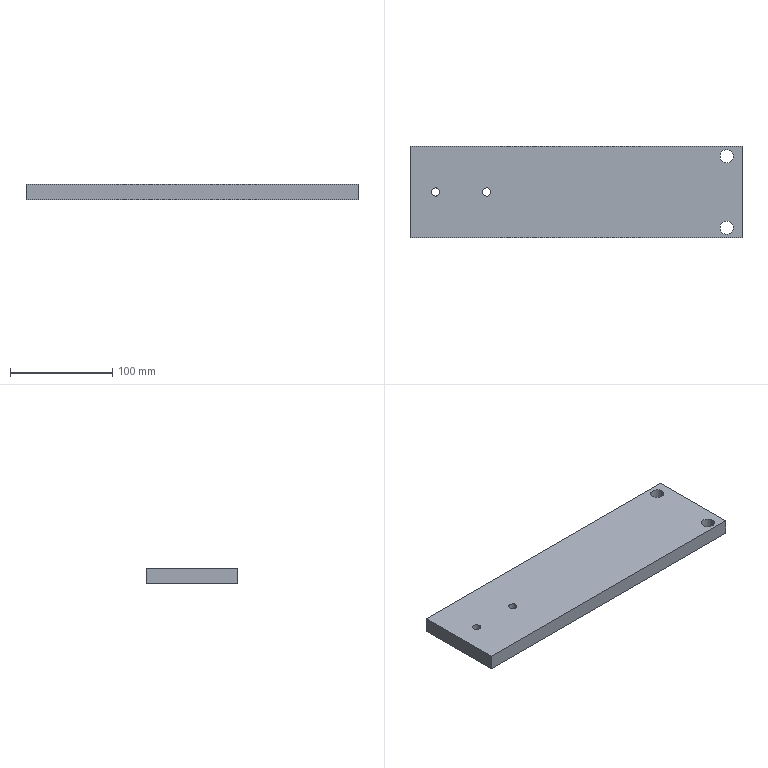Part | NX | features solid 2 | 1 solid | 10 faces | box 325 x 90 x 15 mm | volume 433260 mm3 | plane 6 | cylinder 4 | commonest cylinder face diameters 8 x2 13 x2
STEP:
#1=CARTESIAN_POINT('',(-351.,-440.,-110.));
#2=VERTEX_POINT('',#1);
#3=CARTESIAN_POINT('',(-355.,-440.,-110.));
#4=DIRECTION('',(0.,0.,1.));
#5=DIRECTION('',(1.,0.,0.));
#6=AXIS2_PLACEMENT_3D('',#3,#4,#5);
#7=CIRCLE('',#6,4.);
#8=EDGE_CURVE('',#2,#2,#7,.T.);
#9=ORIENTED_EDGE('',*,*,#8,.F.);
#10=EDGE_LOOP('',(#9));
#11=FACE_BOUND('',#10,.T.);
#12=CARTESIAN_POINT('',(-401.,-440.,-110.));
#13=VERTEX_POINT('',#12);
#14=CARTESIAN_POINT('',(-405.,-440.,-110.));
#15=DIRECTION('',(0.,0.,1.));
#16=DIRECTION('',(1.,0.,0.));
#17=AXIS2_PLACEMENT_3D('',#14,#15,#16);
#18=CIRCLE('',#17,4.);
#19=EDGE_CURVE('',#13,#13,#18,.T.);
#20=ORIENTED_EDGE('',*,*,#19,.F.);
#21=EDGE_LOOP('',(#20));
#22=FACE_BOUND('',#21,.T.);
#23=CARTESIAN_POINT('',(-113.5,-405.,-110.));
#24=VERTEX_POINT('',#23);
#25=CARTESIAN_POINT('',(-120.,-405.,-110.));
#26=DIRECTION('',(0.,0.,1.));
#27=DIRECTION('',(1.,0.,0.));
#28=AXIS2_PLACEMENT_3D('',#25,#26,#27);
#29=CIRCLE('',#28,6.5);
#30=EDGE_CURVE('',#24,#24,#29,.T.);
#31=ORIENTED_EDGE('',*,*,#30,.F.);
#32=EDGE_LOOP('',(#31));
#33=FACE_BOUND('',#32,.T.);
#34=CARTESIAN_POINT('',(-430.,-395.,-110.));
#35=VERTEX_POINT('',#34);
#36=CARTESIAN_POINT('',(-105.,-395.,-110.));
#37=VERTEX_POINT('',#36);
#38=CARTESIAN_POINT('',(-485.,-395.,-110.));
#39=DIRECTION('',(-1.,0.,0.));
#40=VECTOR('',#39,1000.);
#41=LINE('',#38,#40);
#42=EDGE_CURVE('',#35,#37,#41,.F.);
#43=ORIENTED_EDGE('',*,*,#42,.F.);
#44=CARTESIAN_POINT('',(-430.,-485.,-110.));
#45=VERTEX_POINT('',#44);
#46=CARTESIAN_POINT('',(-430.,-395.,-110.));
#47=DIRECTION('',(0.,1.,0.));
#48=VECTOR('',#47,1000.);
#49=LINE('',#46,#48);
#50=EDGE_CURVE('',#45,#35,#49,.T.);
#51=ORIENTED_EDGE('',*,*,#50,.F.);
#52=CARTESIAN_POINT('',(-105.,-485.,-110.));
#53=VERTEX_POINT('',#52);
#54=CARTESIAN_POINT('',(-485.,-485.,-110.));
#55=DIRECTION('',(1.,0.,0.));
#56=VECTOR('',#55,1000.);
#57=LINE('',#54,#56);
#58=EDGE_CURVE('',#45,#53,#57,.T.);
#59=ORIENTED_EDGE('',*,*,#58,.T.);
#60=CARTESIAN_POINT('',(-105.,-775.,-110.));
#61=DIRECTION('',(0.,-1.,0.));
#62=VECTOR('',#61,1000.);
#63=LINE('',#60,#62);
#64=EDGE_CURVE('',#37,#53,#63,.T.);
#65=ORIENTED_EDGE('',*,*,#64,.F.);
#66=EDGE_LOOP('',(#43,#51,#59,#65));
#67=FACE_BOUND('',#66,.T.);
#68=CARTESIAN_POINT('',(-113.5,-475.,-110.));
#69=VERTEX_POINT('',#68);
#70=CARTESIAN_POINT('',(-120.,-475.,-110.));
#71=DIRECTION('',(0.,0.,1.));
#72=DIRECTION('',(1.,0.,0.));
#73=AXIS2_PLACEMENT_3D('',#70,#71,#72);
#74=CIRCLE('',#73,6.5);
#75=EDGE_CURVE('',#69,#69,#74,.F.);
#76=ORIENTED_EDGE('',*,*,#75,.T.);
#77=EDGE_LOOP('',(#76));
#78=FACE_BOUND('',#77,.T.);
#79=CARTESIAN_POINT('',(-485.,-775.,-110.));
#80=DIRECTION('',(0.,0.,1.));
#81=DIRECTION('',(-1.,0.,0.));
#82=AXIS2_PLACEMENT_3D('',#79,#80,#81);
#83=PLANE('',#82);
#84=ADVANCED_FACE('',(#11,#22,#33,#67,#78),#83,.T.);
#85=CARTESIAN_POINT('',(-351.,-440.,-125.));
#86=VERTEX_POINT('',#85);
#87=CARTESIAN_POINT('',(-355.,-440.,-125.));
#88=DIRECTION('',(0.,0.,1.));
#89=DIRECTION('',(1.,0.,0.));
#90=AXIS2_PLACEMENT_3D('',#87,#88,#89);
#91=CIRCLE('',#90,4.);
#92=EDGE_CURVE('',#86,#86,#91,.T.);
#93=ORIENTED_EDGE('',*,*,#92,.T.);
#94=EDGE_LOOP('',(#93));
#95=FACE_BOUND('',#94,.T.);
#96=CARTESIAN_POINT('',(-401.,-440.,-125.));
#97=VERTEX_POINT('',#96);
#98=CARTESIAN_POINT('',(-405.,-440.,-125.));
#99=DIRECTION('',(0.,0.,1.));
#100=DIRECTION('',(1.,0.,0.));
#101=AXIS2_PLACEMENT_3D('',#98,#99,#100);
#102=CIRCLE('',#101,4.);
#103=EDGE_CURVE('',#97,#97,#102,.T.);
#104=ORIENTED_EDGE('',*,*,#103,.T.);
#105=EDGE_LOOP('',(#104));
#106=FACE_BOUND('',#105,.T.);
#107=CARTESIAN_POINT('',(-126.5,-405.,-125.));
#108=VERTEX_POINT('',#107);
#109=CARTESIAN_POINT('',(-120.,-405.,-125.));
#110=DIRECTION('',(0.,0.,-1.));
#111=DIRECTION('',(-1.,0.,0.));
#112=AXIS2_PLACEMENT_3D('',#109,#110,#111);
#113=CIRCLE('',#112,6.5);
#114=EDGE_CURVE('',#108,#108,#113,.F.);
#115=ORIENTED_EDGE('',*,*,#114,.T.);
#116=EDGE_LOOP('',(#115));
#117=FACE_BOUND('',#116,.T.);
#118=CARTESIAN_POINT('',(-105.,-395.,-125.));
#119=VERTEX_POINT('',#118);
#120=CARTESIAN_POINT('',(-105.,-485.,-125.));
#121=VERTEX_POINT('',#120);
#122=CARTESIAN_POINT('',(-105.,-435.,-125.));
#123=DIRECTION('',(0.,1.,0.));
#124=VECTOR('',#123,1000.);
#125=LINE('',#122,#124);
#126=EDGE_CURVE('',#119,#121,#125,.F.);
#127=ORIENTED_EDGE('',*,*,#126,.T.);
#128=CARTESIAN_POINT('',(-430.,-485.,-125.));
#129=VERTEX_POINT('',#128);
#130=CARTESIAN_POINT('',(-135.,-485.,-125.));
#131=DIRECTION('',(-1.,0.,0.));
#132=VECTOR('',#131,1000.);
#133=LINE('',#130,#132);
#134=EDGE_CURVE('',#129,#121,#133,.F.);
#135=ORIENTED_EDGE('',*,*,#134,.F.);
#136=CARTESIAN_POINT('',(-430.,-395.,-125.));
#137=VERTEX_POINT('',#136);
#138=CARTESIAN_POINT('',(-430.,-395.,-125.));
#139=DIRECTION('',(0.,-1.,0.));
#140=VECTOR('',#139,1000.);
#141=LINE('',#138,#140);
#142=EDGE_CURVE('',#129,#137,#141,.F.);
#143=ORIENTED_EDGE('',*,*,#142,.T.);
#144=CARTESIAN_POINT('',(-135.,-395.,-125.));
#145=DIRECTION('',(1.,0.,0.));
#146=VECTOR('',#145,1000.);
#147=LINE('',#144,#146);
#148=EDGE_CURVE('',#137,#119,#147,.T.);
#149=ORIENTED_EDGE('',*,*,#148,.T.);
#150=EDGE_LOOP('',(#127,#135,#143,#149));
#151=FACE_BOUND('',#150,.T.);
#152=CARTESIAN_POINT('',(-126.5,-475.,-125.));
#153=VERTEX_POINT('',#152);
#154=CARTESIAN_POINT('',(-120.,-475.,-125.));
#155=DIRECTION('',(0.,0.,-1.));
#156=DIRECTION('',(-1.,0.,0.));
#157=AXIS2_PLACEMENT_3D('',#154,#155,#156);
#158=CIRCLE('',#157,6.5);
#159=EDGE_CURVE('',#153,#153,#158,.T.);
#160=ORIENTED_EDGE('',*,*,#159,.F.);
#161=EDGE_LOOP('',(#160));
#162=FACE_BOUND('',#161,.T.);
#163=CARTESIAN_POINT('',(-135.,-435.,-125.));
#164=DIRECTION('',(0.,0.,-1.));
#165=DIRECTION('',(0.,-1.,0.));
#166=AXIS2_PLACEMENT_3D('',#163,#164,#165);
#167=PLANE('',#166);
#168=ADVANCED_FACE('',(#95,#106,#117,#151,#162),#167,.T.);
#169=ORIENTED_EDGE('',*,*,#64,.T.);
#170=CARTESIAN_POINT('',(-105.,-485.,-125.));
#171=DIRECTION('',(0.,0.,-1.));
#172=VECTOR('',#171,1000.);
#173=LINE('',#170,#172);
#174=EDGE_CURVE('',#53,#121,#173,.T.);
#175=ORIENTED_EDGE('',*,*,#174,.T.);
#176=ORIENTED_EDGE('',*,*,#126,.F.);
#177=CARTESIAN_POINT('',(-105.,-395.,-125.));
#178=DIRECTION('',(0.,0.,1.));
#179=VECTOR('',#178,1000.);
#180=LINE('',#177,#179);
#181=EDGE_CURVE('',#37,#119,#180,.F.);
#182=ORIENTED_EDGE('',*,*,#181,.F.);
#183=EDGE_LOOP('',(#169,#175,#176,#182));
#184=FACE_BOUND('',#183,.T.);
#185=CARTESIAN_POINT('',(-105.,-395.,-125.));
#186=DIRECTION('',(1.,0.,0.));
#187=DIRECTION('',(0.,0.,1.));
#188=AXIS2_PLACEMENT_3D('',#185,#186,#187);
#189=PLANE('',#188);
#190=ADVANCED_FACE('',(#184),#189,.T.);
#191=ORIENTED_EDGE('',*,*,#181,.T.);
#192=ORIENTED_EDGE('',*,*,#148,.F.);
#193=CARTESIAN_POINT('',(-430.,-395.,-204.));
#194=DIRECTION('',(0.,0.,-1.));
#195=VECTOR('',#194,1000.);
#196=LINE('',#193,#195);
#197=EDGE_CURVE('',#137,#35,#196,.F.);
#198=ORIENTED_EDGE('',*,*,#197,.T.);
#199=ORIENTED_EDGE('',*,*,#42,.T.);
#200=EDGE_LOOP('',(#191,#192,#198,#199));
#201=FACE_BOUND('',#200,.T.);
#202=CARTESIAN_POINT('',(-135.,-395.,-144.));
#203=DIRECTION('',(0.,1.,0.));
#204=DIRECTION('',(0.,0.,-1.));
#205=AXIS2_PLACEMENT_3D('',#202,#203,#204);
#206=PLANE('',#205);
#207=ADVANCED_FACE('',(#201),#206,.T.);
#208=ORIENTED_EDGE('',*,*,#58,.F.);
#209=CARTESIAN_POINT('',(-430.,-485.,-204.));
#210=DIRECTION('',(0.,0.,1.));
#211=VECTOR('',#210,1000.);
#212=LINE('',#209,#211);
#213=EDGE_CURVE('',#129,#45,#212,.T.);
#214=ORIENTED_EDGE('',*,*,#213,.F.);
#215=ORIENTED_EDGE('',*,*,#134,.T.);
#216=ORIENTED_EDGE('',*,*,#174,.F.);
#217=EDGE_LOOP('',(#208,#214,#215,#216));
#218=FACE_BOUND('',#217,.T.);
#219=CARTESIAN_POINT('',(135.,-485.,-144.));
#220=DIRECTION('',(0.,-1.,0.));
#221=DIRECTION('',(0.,0.,1.));
#222=AXIS2_PLACEMENT_3D('',#219,#220,#221);
#223=PLANE('',#222);
#224=ADVANCED_FACE('',(#218),#223,.T.);
#225=ORIENTED_EDGE('',*,*,#213,.T.);
#226=ORIENTED_EDGE('',*,*,#50,.T.);
#227=ORIENTED_EDGE('',*,*,#197,.F.);
#228=ORIENTED_EDGE('',*,*,#142,.F.);
#229=EDGE_LOOP('',(#225,#226,#227,#228));
#230=FACE_BOUND('',#229,.T.);
#231=CARTESIAN_POINT('',(-430.,-395.,-204.));
#232=DIRECTION('',(-1.,0.,0.));
#233=DIRECTION('',(0.,0.,1.));
#234=AXIS2_PLACEMENT_3D('',#231,#232,#233);
#235=PLANE('',#234);
#236=ADVANCED_FACE('',(#230),#235,.T.);
#237=ORIENTED_EDGE('',*,*,#75,.F.);
#238=EDGE_LOOP('',(#237));
#239=FACE_BOUND('',#238,.T.);
#240=ORIENTED_EDGE('',*,*,#159,.T.);
#241=EDGE_LOOP('',(#240));
#242=FACE_BOUND('',#241,.T.);
#243=CARTESIAN_POINT('',(-120.,-475.,-94.));
#244=DIRECTION('',(0.,0.,-1.));
#245=DIRECTION('',(-1.,0.,0.));
#246=AXIS2_PLACEMENT_3D('',#243,#244,#245);
#247=CYLINDRICAL_SURFACE('',#246,6.5);
#248=ADVANCED_FACE('',(#239,#242),#247,.F.);
#249=ORIENTED_EDGE('',*,*,#30,.T.);
#250=EDGE_LOOP('',(#249));
#251=FACE_BOUND('',#250,.T.);
#252=ORIENTED_EDGE('',*,*,#114,.F.);
#253=EDGE_LOOP('',(#252));
#254=FACE_BOUND('',#253,.T.);
#255=CARTESIAN_POINT('',(-120.,-405.,-94.));
#256=DIRECTION('',(0.,0.,-1.));
#257=DIRECTION('',(-1.,0.,0.));
#258=AXIS2_PLACEMENT_3D('',#255,#256,#257);
#259=CYLINDRICAL_SURFACE('',#258,6.5);
#260=ADVANCED_FACE('',(#251,#254),#259,.F.);
#261=ORIENTED_EDGE('',*,*,#19,.T.);
#262=EDGE_LOOP('',(#261));
#263=FACE_BOUND('',#262,.T.);
#264=ORIENTED_EDGE('',*,*,#103,.F.);
#265=EDGE_LOOP('',(#264));
#266=FACE_BOUND('',#265,.T.);
#267=CARTESIAN_POINT('',(-405.,-440.,-125.));
#268=DIRECTION('',(0.,0.,1.));
#269=DIRECTION('',(1.,0.,0.));
#270=AXIS2_PLACEMENT_3D('',#267,#268,#269);
#271=CYLINDRICAL_SURFACE('',#270,4.);
#272=ADVANCED_FACE('',(#263,#266),#271,.F.);
#273=ORIENTED_EDGE('',*,*,#8,.T.);
#274=EDGE_LOOP('',(#273));
#275=FACE_BOUND('',#274,.T.);
#276=ORIENTED_EDGE('',*,*,#92,.F.);
#277=EDGE_LOOP('',(#276));
#278=FACE_BOUND('',#277,.T.);
#279=CARTESIAN_POINT('',(-355.,-440.,-125.));
#280=DIRECTION('',(0.,0.,1.));
#281=DIRECTION('',(1.,0.,0.));
#282=AXIS2_PLACEMENT_3D('',#279,#280,#281);
#283=CYLINDRICAL_SURFACE('',#282,4.);
#284=ADVANCED_FACE('',(#275,#278),#283,.F.);
#285=CLOSED_SHELL('',(#84,#168,#190,#207,#224,#236,#248,#260,#272,#284));
#286=MANIFOLD_SOLID_BREP('',#285);
#287=(LENGTH_UNIT()NAMED_UNIT(*)SI_UNIT(.MILLI.,.METRE.));
#288=UNCERTAINTY_MEASURE_WITH_UNIT(LENGTH_MEASURE(0.00001),#287,'','');
#289=(NAMED_UNIT(*)PLANE_ANGLE_UNIT()SI_UNIT($,.RADIAN.));
#290=(NAMED_UNIT(*)SI_UNIT($,.STERADIAN.)SOLID_ANGLE_UNIT());
#291=(GEOMETRIC_REPRESENTATION_CONTEXT(3)GLOBAL_UNCERTAINTY_ASSIGNED_CONTEXT((#288))GLOBAL_UNIT_ASSIGNED_CONTEXT((#287,#289,#290))REPRESENTATION_CONTEXT('',''));
#292=ADVANCED_BREP_SHAPE_REPRESENTATION('',(#286),#291);